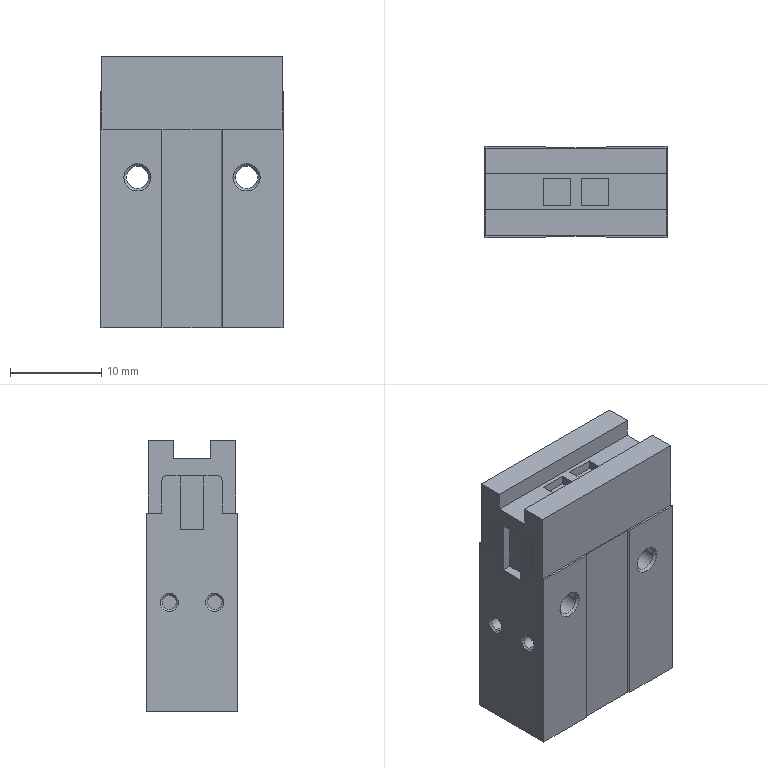Part | STEP file | 1 | 1 solid | 101 faces | box 20 x 10 x 29.8 mm | volume 5405 mm3 | plane 59 | cylinder 22 | cone 20 | commonest cylinder face diameters 1.567 x8 2.459 x8 1 x4 7 x2